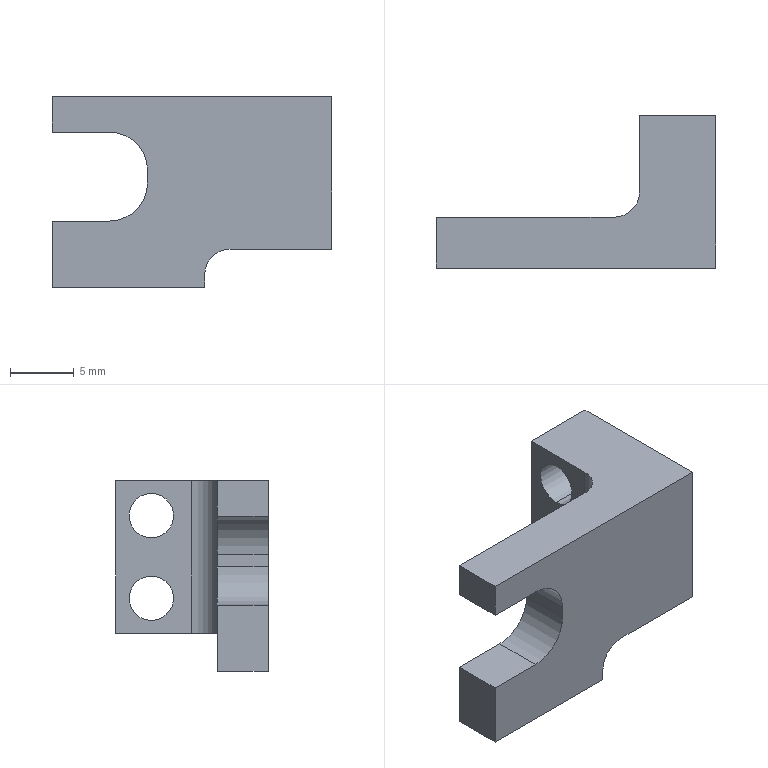Part | NX | features BREP 1 | 1 solid | 22 faces | box 22 x 12 x 15 mm | volume 1480 mm3 | plane 14 | cylinder 8 | commonest cylinder face diameters 3.5 x4 4 x2 6 x2
STEP:
#1=CARTESIAN_POINT('',(-769.249,20.164,1.));
#2=VERTEX_POINT('',#1);
#3=CARTESIAN_POINT('',(-769.249,20.164,4.5));
#4=VERTEX_POINT('',#3);
#5=CARTESIAN_POINT('',(-769.249,20.164,2.75));
#6=DIRECTION('',(-1.,0.,0.));
#7=DIRECTION('',(0.,0.,1.));
#8=AXIS2_PLACEMENT_3D('',#5,#6,#7);
#9=CIRCLE('',#8,1.75);
#10=EDGE_CURVE('',#2,#4,#9,.T.);
#11=ORIENTED_EDGE('',*,*,#10,.F.);
#12=CARTESIAN_POINT('',(-775.249,20.164,1.));
#13=VERTEX_POINT('',#12);
#14=CARTESIAN_POINT('',(-769.249,20.164,1.));
#15=DIRECTION('',(-1.,0.,0.));
#16=VECTOR('',#15,1000.);
#17=LINE('',#14,#16);
#18=EDGE_CURVE('',#13,#2,#17,.F.);
#19=ORIENTED_EDGE('',*,*,#18,.F.);
#20=CARTESIAN_POINT('',(-775.249,20.164,4.5));
#21=VERTEX_POINT('',#20);
#22=CARTESIAN_POINT('',(-775.249,20.164,2.75));
#23=DIRECTION('',(-1.,0.,0.));
#24=DIRECTION('',(0.,0.,1.));
#25=AXIS2_PLACEMENT_3D('',#22,#23,#24);
#26=CIRCLE('',#25,1.75);
#27=EDGE_CURVE('',#13,#21,#26,.T.);
#28=ORIENTED_EDGE('',*,*,#27,.T.);
#29=CARTESIAN_POINT('',(-769.249,20.164,4.5));
#30=DIRECTION('',(-1.,0.,0.));
#31=VECTOR('',#30,1000.);
#32=LINE('',#29,#31);
#33=EDGE_CURVE('',#21,#4,#32,.F.);
#34=ORIENTED_EDGE('',*,*,#33,.T.);
#35=EDGE_LOOP('',(#11,#19,#28,#34));
#36=FACE_BOUND('',#35,.T.);
#37=CARTESIAN_POINT('',(-769.249,20.164,2.75));
#38=DIRECTION('',(-1.,0.,0.));
#39=DIRECTION('',(0.,0.,1.));
#40=AXIS2_PLACEMENT_3D('',#37,#38,#39);
#41=CYLINDRICAL_SURFACE('',#40,1.75);
#42=ADVANCED_FACE('',(#36),#41,.F.);
#43=CARTESIAN_POINT('',(-769.249,20.164,7.5));
#44=VERTEX_POINT('',#43);
#45=CARTESIAN_POINT('',(-769.249,20.164,11.));
#46=VERTEX_POINT('',#45);
#47=CARTESIAN_POINT('',(-769.249,20.164,9.25));
#48=DIRECTION('',(-1.,0.,0.));
#49=DIRECTION('',(0.,0.,1.));
#50=AXIS2_PLACEMENT_3D('',#47,#48,#49);
#51=CIRCLE('',#50,1.75);
#52=EDGE_CURVE('',#44,#46,#51,.T.);
#53=ORIENTED_EDGE('',*,*,#52,.F.);
#54=CARTESIAN_POINT('',(-775.249,20.164,7.5));
#55=VERTEX_POINT('',#54);
#56=CARTESIAN_POINT('',(-769.249,20.164,7.5));
#57=DIRECTION('',(-1.,0.,0.));
#58=VECTOR('',#57,1000.);
#59=LINE('',#56,#58);
#60=EDGE_CURVE('',#55,#44,#59,.F.);
#61=ORIENTED_EDGE('',*,*,#60,.F.);
#62=CARTESIAN_POINT('',(-775.249,20.164,11.));
#63=VERTEX_POINT('',#62);
#64=CARTESIAN_POINT('',(-775.249,20.164,9.25));
#65=DIRECTION('',(-1.,0.,0.));
#66=DIRECTION('',(0.,0.,1.));
#67=AXIS2_PLACEMENT_3D('',#64,#65,#66);
#68=CIRCLE('',#67,1.75);
#69=EDGE_CURVE('',#55,#63,#68,.T.);
#70=ORIENTED_EDGE('',*,*,#69,.T.);
#71=CARTESIAN_POINT('',(-769.249,20.164,11.));
#72=DIRECTION('',(-1.,0.,0.));
#73=VECTOR('',#72,1000.);
#74=LINE('',#71,#73);
#75=EDGE_CURVE('',#63,#46,#74,.F.);
#76=ORIENTED_EDGE('',*,*,#75,.T.);
#77=EDGE_LOOP('',(#53,#61,#70,#76));
#78=FACE_BOUND('',#77,.T.);
#79=CARTESIAN_POINT('',(-769.249,20.164,9.25));
#80=DIRECTION('',(-1.,0.,0.));
#81=DIRECTION('',(0.,0.,1.));
#82=AXIS2_PLACEMENT_3D('',#79,#80,#81);
#83=CYLINDRICAL_SURFACE('',#82,1.75);
#84=ADVANCED_FACE('',(#78),#83,.F.);
#85=CARTESIAN_POINT('',(-791.249,10.964,9.213));
#86=VERTEX_POINT('',#85);
#87=CARTESIAN_POINT('',(-791.249,14.964,9.213));
#88=VERTEX_POINT('',#87);
#89=CARTESIAN_POINT('',(-791.249,14.964,9.213));
#90=DIRECTION('',(0.,1.,0.));
#91=VECTOR('',#90,1000.);
#92=LINE('',#89,#91);
#93=EDGE_CURVE('',#86,#88,#92,.T.);
#94=ORIENTED_EDGE('',*,*,#93,.F.);
#95=CARTESIAN_POINT('',(-791.249,10.964,12.));
#96=VERTEX_POINT('',#95);
#97=CARTESIAN_POINT('',(-791.249,10.964,12.));
#98=DIRECTION('',(0.,0.,1.));
#99=VECTOR('',#98,1000.);
#100=LINE('',#97,#99);
#101=EDGE_CURVE('',#86,#96,#100,.T.);
#102=ORIENTED_EDGE('',*,*,#101,.T.);
#103=CARTESIAN_POINT('',(-791.249,14.964,12.));
#104=VERTEX_POINT('',#103);
#105=CARTESIAN_POINT('',(-791.249,10.964,12.));
#106=DIRECTION('',(0.,1.,0.));
#107=VECTOR('',#106,1000.);
#108=LINE('',#105,#107);
#109=EDGE_CURVE('',#96,#104,#108,.T.);
#110=ORIENTED_EDGE('',*,*,#109,.T.);
#111=CARTESIAN_POINT('',(-791.249,14.964,12.));
#112=DIRECTION('',(0.,0.,-1.));
#113=VECTOR('',#112,1000.);
#114=LINE('',#111,#113);
#115=EDGE_CURVE('',#104,#88,#114,.T.);
#116=ORIENTED_EDGE('',*,*,#115,.T.);
#117=EDGE_LOOP('',(#94,#102,#110,#116));
#118=FACE_BOUND('',#117,.T.);
#119=CARTESIAN_POINT('',(-791.249,14.964,12.));
#120=DIRECTION('',(-1.,0.,0.));
#121=DIRECTION('',(0.,0.,1.));
#122=AXIS2_PLACEMENT_3D('',#119,#120,#121);
#123=PLANE('',#122);
#124=ADVANCED_FACE('',(#118),#123,.T.);
#125=CARTESIAN_POINT('',(-777.249,10.964,0.));
#126=VERTEX_POINT('',#125);
#127=CARTESIAN_POINT('',(-769.249,10.964,0.));
#128=VERTEX_POINT('',#127);
#129=CARTESIAN_POINT('',(-769.249,10.964,0.));
#130=DIRECTION('',(1.,0.,0.));
#131=VECTOR('',#130,1000.);
#132=LINE('',#129,#131);
#133=EDGE_CURVE('',#126,#128,#132,.T.);
#134=ORIENTED_EDGE('',*,*,#133,.F.);
#135=CARTESIAN_POINT('',(-777.249,14.964,0.));
#136=VERTEX_POINT('',#135);
#137=CARTESIAN_POINT('',(-777.249,14.964,0.));
#138=DIRECTION('',(0.,1.,0.));
#139=VECTOR('',#138,1000.);
#140=LINE('',#137,#139);
#141=EDGE_CURVE('',#126,#136,#140,.T.);
#142=ORIENTED_EDGE('',*,*,#141,.T.);
#143=CARTESIAN_POINT('',(-775.249,16.964,0.));
#144=VERTEX_POINT('',#143);
#145=CARTESIAN_POINT('',(-777.249,16.964,0.));
#146=DIRECTION('',(0.,0.,1.));
#147=DIRECTION('',(-1.,0.,0.));
#148=AXIS2_PLACEMENT_3D('',#145,#146,#147);
#149=CIRCLE('',#148,2.);
#150=EDGE_CURVE('',#136,#144,#149,.T.);
#151=ORIENTED_EDGE('',*,*,#150,.T.);
#152=CARTESIAN_POINT('',(-775.249,22.964,0.));
#153=VERTEX_POINT('',#152);
#154=CARTESIAN_POINT('',(-775.249,22.964,0.));
#155=DIRECTION('',(0.,-1.,0.));
#156=VECTOR('',#155,1000.);
#157=LINE('',#154,#156);
#158=EDGE_CURVE('',#153,#144,#157,.T.);
#159=ORIENTED_EDGE('',*,*,#158,.F.);
#160=CARTESIAN_POINT('',(-769.249,22.964,0.));
#161=VERTEX_POINT('',#160);
#162=CARTESIAN_POINT('',(-769.249,22.964,0.));
#163=DIRECTION('',(-1.,0.,0.));
#164=VECTOR('',#163,1000.);
#165=LINE('',#162,#164);
#166=EDGE_CURVE('',#161,#153,#165,.T.);
#167=ORIENTED_EDGE('',*,*,#166,.F.);
#168=CARTESIAN_POINT('',(-769.249,22.964,0.));
#169=DIRECTION('',(0.,1.,0.));
#170=VECTOR('',#169,1000.);
#171=LINE('',#168,#170);
#172=EDGE_CURVE('',#128,#161,#171,.T.);
#173=ORIENTED_EDGE('',*,*,#172,.F.);
#174=EDGE_LOOP('',(#134,#142,#151,#159,#167,#173));
#175=FACE_BOUND('',#174,.T.);
#176=CARTESIAN_POINT('',(-769.249,10.964,0.));
#177=DIRECTION('',(0.,0.,-1.));
#178=DIRECTION('',(0.,-1.,0.));
#179=AXIS2_PLACEMENT_3D('',#176,#177,#178);
#180=PLANE('',#179);
#181=ADVANCED_FACE('',(#175),#180,.T.);
#182=ORIENTED_EDGE('',*,*,#158,.T.);
#183=CARTESIAN_POINT('',(-775.249,16.964,12.));
#184=VERTEX_POINT('',#183);
#185=CARTESIAN_POINT('',(-775.249,16.964,12.));
#186=DIRECTION('',(0.,0.,1.));
#187=VECTOR('',#186,1000.);
#188=LINE('',#185,#187);
#189=EDGE_CURVE('',#144,#184,#188,.T.);
#190=ORIENTED_EDGE('',*,*,#189,.T.);
#191=CARTESIAN_POINT('',(-775.249,22.964,12.));
#192=VERTEX_POINT('',#191);
#193=CARTESIAN_POINT('',(-775.249,22.964,12.));
#194=DIRECTION('',(0.,-1.,0.));
#195=VECTOR('',#194,1000.);
#196=LINE('',#193,#195);
#197=EDGE_CURVE('',#192,#184,#196,.T.);
#198=ORIENTED_EDGE('',*,*,#197,.F.);
#199=CARTESIAN_POINT('',(-775.249,22.964,12.));
#200=DIRECTION('',(0.,0.,-1.));
#201=VECTOR('',#200,1000.);
#202=LINE('',#199,#201);
#203=EDGE_CURVE('',#192,#153,#202,.T.);
#204=ORIENTED_EDGE('',*,*,#203,.T.);
#205=EDGE_LOOP('',(#182,#190,#198,#204));
#206=FACE_BOUND('',#205,.T.);
#207=CARTESIAN_POINT('',(-775.249,20.164,2.75));
#208=DIRECTION('',(-1.,0.,0.));
#209=DIRECTION('',(0.,0.,1.));
#210=AXIS2_PLACEMENT_3D('',#207,#208,#209);
#211=CIRCLE('',#210,1.75);
#212=EDGE_CURVE('',#21,#13,#211,.T.);
#213=ORIENTED_EDGE('',*,*,#212,.F.);
#214=ORIENTED_EDGE('',*,*,#27,.F.);
#215=EDGE_LOOP('',(#213,#214));
#216=FACE_BOUND('',#215,.T.);
#217=CARTESIAN_POINT('',(-775.249,20.164,9.25));
#218=DIRECTION('',(-1.,0.,0.));
#219=DIRECTION('',(0.,0.,1.));
#220=AXIS2_PLACEMENT_3D('',#217,#218,#219);
#221=CIRCLE('',#220,1.75);
#222=EDGE_CURVE('',#63,#55,#221,.T.);
#223=ORIENTED_EDGE('',*,*,#222,.F.);
#224=ORIENTED_EDGE('',*,*,#69,.F.);
#225=EDGE_LOOP('',(#223,#224));
#226=FACE_BOUND('',#225,.T.);
#227=CARTESIAN_POINT('',(-775.249,22.964,12.));
#228=DIRECTION('',(1.,0.,0.));
#229=DIRECTION('',(0.,1.,0.));
#230=AXIS2_PLACEMENT_3D('',#227,#228,#229);
#231=PLANE('',#230);
#232=ADVANCED_FACE('',(#206,#216,#226),#231,.F.);
#233=ORIENTED_EDGE('',*,*,#172,.T.);
#234=CARTESIAN_POINT('',(-769.249,22.964,12.));
#235=VERTEX_POINT('',#234);
#236=CARTESIAN_POINT('',(-769.249,22.964,12.));
#237=DIRECTION('',(0.,0.,-1.));
#238=VECTOR('',#237,1000.);
#239=LINE('',#236,#238);
#240=EDGE_CURVE('',#235,#161,#239,.T.);
#241=ORIENTED_EDGE('',*,*,#240,.F.);
#242=CARTESIAN_POINT('',(-769.249,10.964,12.));
#243=VERTEX_POINT('',#242);
#244=CARTESIAN_POINT('',(-769.249,22.964,12.));
#245=DIRECTION('',(0.,1.,0.));
#246=VECTOR('',#245,1000.);
#247=LINE('',#244,#246);
#248=EDGE_CURVE('',#243,#235,#247,.T.);
#249=ORIENTED_EDGE('',*,*,#248,.F.);
#250=CARTESIAN_POINT('',(-769.249,10.964,12.));
#251=DIRECTION('',(0.,0.,-1.));
#252=VECTOR('',#251,1000.);
#253=LINE('',#250,#252);
#254=EDGE_CURVE('',#243,#128,#253,.T.);
#255=ORIENTED_EDGE('',*,*,#254,.T.);
#256=EDGE_LOOP('',(#233,#241,#249,#255));
#257=FACE_BOUND('',#256,.T.);
#258=CARTESIAN_POINT('',(-769.249,20.164,2.75));
#259=DIRECTION('',(-1.,0.,0.));
#260=DIRECTION('',(0.,0.,1.));
#261=AXIS2_PLACEMENT_3D('',#258,#259,#260);
#262=CIRCLE('',#261,1.75);
#263=EDGE_CURVE('',#4,#2,#262,.T.);
#264=ORIENTED_EDGE('',*,*,#263,.T.);
#265=ORIENTED_EDGE('',*,*,#10,.T.);
#266=EDGE_LOOP('',(#264,#265));
#267=FACE_BOUND('',#266,.T.);
#268=CARTESIAN_POINT('',(-769.249,20.164,9.25));
#269=DIRECTION('',(-1.,0.,0.));
#270=DIRECTION('',(0.,0.,1.));
#271=AXIS2_PLACEMENT_3D('',#268,#269,#270);
#272=CIRCLE('',#271,1.75);
#273=EDGE_CURVE('',#46,#44,#272,.T.);
#274=ORIENTED_EDGE('',*,*,#273,.T.);
#275=ORIENTED_EDGE('',*,*,#52,.T.);
#276=EDGE_LOOP('',(#274,#275));
#277=FACE_BOUND('',#276,.T.);
#278=CARTESIAN_POINT('',(-769.249,22.964,12.));
#279=DIRECTION('',(-1.,0.,0.));
#280=DIRECTION('',(0.,0.,1.));
#281=AXIS2_PLACEMENT_3D('',#278,#279,#280);
#282=PLANE('',#281);
#283=ADVANCED_FACE('',(#257,#267,#277),#282,.F.);
#284=ORIENTED_EDGE('',*,*,#166,.T.);
#285=ORIENTED_EDGE('',*,*,#203,.F.);
#286=CARTESIAN_POINT('',(-769.249,22.964,12.));
#287=DIRECTION('',(-1.,0.,0.));
#288=VECTOR('',#287,1000.);
#289=LINE('',#286,#288);
#290=EDGE_CURVE('',#235,#192,#289,.T.);
#291=ORIENTED_EDGE('',*,*,#290,.F.);
#292=ORIENTED_EDGE('',*,*,#240,.T.);
#293=EDGE_LOOP('',(#284,#285,#291,#292));
#294=FACE_BOUND('',#293,.T.);
#295=CARTESIAN_POINT('',(-769.249,22.964,12.));
#296=DIRECTION('',(0.,-1.,0.));
#297=DIRECTION('',(0.,0.,-1.));
#298=AXIS2_PLACEMENT_3D('',#295,#296,#297);
#299=PLANE('',#298);
#300=ADVANCED_FACE('',(#294),#299,.F.);
#301=ORIENTED_EDGE('',*,*,#101,.F.);
#302=CARTESIAN_POINT('',(-786.749,10.964,9.213));
#303=VERTEX_POINT('',#302);
#304=CARTESIAN_POINT('',(-769.249,10.964,9.213));
#305=DIRECTION('',(1.,0.,0.));
#306=VECTOR('',#305,1000.);
#307=LINE('',#304,#306);
#308=EDGE_CURVE('',#86,#303,#307,.T.);
#309=ORIENTED_EDGE('',*,*,#308,.T.);
#310=CARTESIAN_POINT('',(-783.749,10.964,6.213));
#311=VERTEX_POINT('',#310);
#312=CARTESIAN_POINT('',(-786.749,10.964,6.213));
#313=DIRECTION('',(0.,1.,0.));
#314=DIRECTION('',(-1.,0.,0.));
#315=AXIS2_PLACEMENT_3D('',#312,#313,#314);
#316=CIRCLE('',#315,3.);
#317=EDGE_CURVE('',#303,#311,#316,.T.);
#318=ORIENTED_EDGE('',*,*,#317,.T.);
#319=CARTESIAN_POINT('',(-783.749,10.964,5.213));
#320=VERTEX_POINT('',#319);
#321=CARTESIAN_POINT('',(-783.749,10.964,12.));
#322=DIRECTION('',(0.,0.,-1.));
#323=VECTOR('',#322,1000.);
#324=LINE('',#321,#323);
#325=EDGE_CURVE('',#311,#320,#324,.T.);
#326=ORIENTED_EDGE('',*,*,#325,.T.);
#327=CARTESIAN_POINT('',(-786.749,10.964,2.213));
#328=VERTEX_POINT('',#327);
#329=CARTESIAN_POINT('',(-786.749,10.964,5.213));
#330=DIRECTION('',(0.,1.,0.));
#331=DIRECTION('',(-1.,0.,0.));
#332=AXIS2_PLACEMENT_3D('',#329,#330,#331);
#333=CIRCLE('',#332,3.);
#334=EDGE_CURVE('',#320,#328,#333,.T.);
#335=ORIENTED_EDGE('',*,*,#334,.T.);
#336=CARTESIAN_POINT('',(-791.249,10.964,2.213));
#337=VERTEX_POINT('',#336);
#338=CARTESIAN_POINT('',(-769.249,10.964,2.213));
#339=DIRECTION('',(-1.,0.,0.));
#340=VECTOR('',#339,1000.);
#341=LINE('',#338,#340);
#342=EDGE_CURVE('',#328,#337,#341,.T.);
#343=ORIENTED_EDGE('',*,*,#342,.T.);
#344=CARTESIAN_POINT('',(-791.249,10.964,-3.));
#345=VERTEX_POINT('',#344);
#346=CARTESIAN_POINT('',(-791.249,10.964,12.));
#347=DIRECTION('',(0.,0.,1.));
#348=VECTOR('',#347,1000.);
#349=LINE('',#346,#348);
#350=EDGE_CURVE('',#345,#337,#349,.T.);
#351=ORIENTED_EDGE('',*,*,#350,.F.);
#352=CARTESIAN_POINT('',(-779.249,10.964,-3.));
#353=VERTEX_POINT('',#352);
#354=CARTESIAN_POINT('',(-791.249,10.964,-3.));
#355=DIRECTION('',(1.,0.,0.));
#356=VECTOR('',#355,1000.);
#357=LINE('',#354,#356);
#358=EDGE_CURVE('',#345,#353,#357,.T.);
#359=ORIENTED_EDGE('',*,*,#358,.T.);
#360=CARTESIAN_POINT('',(-779.249,10.964,-2.));
#361=VERTEX_POINT('',#360);
#362=CARTESIAN_POINT('',(-779.249,10.964,0.));
#363=DIRECTION('',(0.,0.,1.));
#364=VECTOR('',#363,1000.);
#365=LINE('',#362,#364);
#366=EDGE_CURVE('',#353,#361,#365,.T.);
#367=ORIENTED_EDGE('',*,*,#366,.T.);
#368=CARTESIAN_POINT('',(-777.249,10.964,-2.));
#369=DIRECTION('',(0.,1.,0.));
#370=DIRECTION('',(-1.,0.,0.));
#371=AXIS2_PLACEMENT_3D('',#368,#369,#370);
#372=CIRCLE('',#371,2.);
#373=EDGE_CURVE('',#361,#126,#372,.T.);
#374=ORIENTED_EDGE('',*,*,#373,.T.);
#375=ORIENTED_EDGE('',*,*,#133,.T.);
#376=ORIENTED_EDGE('',*,*,#254,.F.);
#377=CARTESIAN_POINT('',(-769.249,10.964,12.));
#378=DIRECTION('',(1.,0.,0.));
#379=VECTOR('',#378,1000.);
#380=LINE('',#377,#379);
#381=EDGE_CURVE('',#96,#243,#380,.T.);
#382=ORIENTED_EDGE('',*,*,#381,.F.);
#383=EDGE_LOOP('',(#301,#309,#318,#326,#335,#343,#351,#359,#367,#374,#375,#376,#382));
#384=FACE_BOUND('',#383,.T.);
#385=CARTESIAN_POINT('',(-769.249,10.964,12.));
#386=DIRECTION('',(0.,1.,0.));
#387=DIRECTION('',(1.,0.,0.));
#388=AXIS2_PLACEMENT_3D('',#385,#386,#387);
#389=PLANE('',#388);
#390=ADVANCED_FACE('',(#384),#389,.F.);
#391=ORIENTED_EDGE('',*,*,#248,.T.);
#392=ORIENTED_EDGE('',*,*,#290,.T.);
#393=ORIENTED_EDGE('',*,*,#197,.T.);
#394=CARTESIAN_POINT('',(-777.249,14.964,12.));
#395=VERTEX_POINT('',#394);
#396=CARTESIAN_POINT('',(-777.249,16.964,12.));
#397=DIRECTION('',(0.,0.,-1.));
#398=DIRECTION('',(-1.,0.,0.));
#399=AXIS2_PLACEMENT_3D('',#396,#397,#398);
#400=CIRCLE('',#399,2.);
#401=EDGE_CURVE('',#184,#395,#400,.T.);
#402=ORIENTED_EDGE('',*,*,#401,.T.);
#403=CARTESIAN_POINT('',(-791.249,14.964,12.));
#404=DIRECTION('',(1.,0.,0.));
#405=VECTOR('',#404,1000.);
#406=LINE('',#403,#405);
#407=EDGE_CURVE('',#104,#395,#406,.T.);
#408=ORIENTED_EDGE('',*,*,#407,.F.);
#409=ORIENTED_EDGE('',*,*,#109,.F.);
#410=ORIENTED_EDGE('',*,*,#381,.T.);
#411=EDGE_LOOP('',(#391,#392,#393,#402,#408,#409,#410));
#412=FACE_BOUND('',#411,.T.);
#413=CARTESIAN_POINT('',(-769.249,10.964,12.));
#414=DIRECTION('',(0.,0.,-1.));
#415=DIRECTION('',(0.,-1.,0.));
#416=AXIS2_PLACEMENT_3D('',#413,#414,#415);
#417=PLANE('',#416);
#418=ADVANCED_FACE('',(#412),#417,.F.);
#419=CARTESIAN_POINT('',(-783.749,14.964,6.213));
#420=VERTEX_POINT('',#419);
#421=CARTESIAN_POINT('',(-783.749,14.964,5.213));
#422=VERTEX_POINT('',#421);
#423=CARTESIAN_POINT('',(-783.749,14.964,9.213));
#424=DIRECTION('',(0.,0.,-1.));
#425=VECTOR('',#424,1000.);
#426=LINE('',#423,#425);
#427=EDGE_CURVE('',#420,#422,#426,.T.);
#428=ORIENTED_EDGE('',*,*,#427,.F.);
#429=CARTESIAN_POINT('',(-786.749,14.964,9.213));
#430=VERTEX_POINT('',#429);
#431=CARTESIAN_POINT('',(-786.749,14.964,6.213));
#432=DIRECTION('',(0.,-1.,0.));
#433=DIRECTION('',(0.,0.,-1.));
#434=AXIS2_PLACEMENT_3D('',#431,#432,#433);
#435=CIRCLE('',#434,3.);
#436=EDGE_CURVE('',#420,#430,#435,.T.);
#437=ORIENTED_EDGE('',*,*,#436,.T.);
#438=CARTESIAN_POINT('',(-783.749,14.964,9.213));
#439=DIRECTION('',(1.,0.,0.));
#440=VECTOR('',#439,1000.);
#441=LINE('',#438,#440);
#442=EDGE_CURVE('',#88,#430,#441,.T.);
#443=ORIENTED_EDGE('',*,*,#442,.F.);
#444=ORIENTED_EDGE('',*,*,#115,.F.);
#445=ORIENTED_EDGE('',*,*,#407,.T.);
#446=CARTESIAN_POINT('',(-777.249,14.964,0.));
#447=DIRECTION('',(0.,0.,-1.));
#448=VECTOR('',#447,1000.);
#449=LINE('',#446,#448);
#450=EDGE_CURVE('',#395,#136,#449,.T.);
#451=ORIENTED_EDGE('',*,*,#450,.T.);
#452=CARTESIAN_POINT('',(-779.249,14.964,-2.));
#453=VERTEX_POINT('',#452);
#454=CARTESIAN_POINT('',(-777.249,14.964,-2.));
#455=DIRECTION('',(0.,-1.,0.));
#456=DIRECTION('',(0.,0.,-1.));
#457=AXIS2_PLACEMENT_3D('',#454,#455,#456);
#458=CIRCLE('',#457,2.);
#459=EDGE_CURVE('',#136,#453,#458,.T.);
#460=ORIENTED_EDGE('',*,*,#459,.T.);
#461=CARTESIAN_POINT('',(-779.249,14.964,-3.));
#462=VERTEX_POINT('',#461);
#463=CARTESIAN_POINT('',(-779.249,14.964,0.));
#464=DIRECTION('',(0.,0.,-1.));
#465=VECTOR('',#464,1000.);
#466=LINE('',#463,#465);
#467=EDGE_CURVE('',#453,#462,#466,.T.);
#468=ORIENTED_EDGE('',*,*,#467,.T.);
#469=CARTESIAN_POINT('',(-791.249,14.964,-3.));
#470=VERTEX_POINT('',#469);
#471=CARTESIAN_POINT('',(-791.249,14.964,-3.));
#472=DIRECTION('',(-1.,0.,0.));
#473=VECTOR('',#472,1000.);
#474=LINE('',#471,#473);
#475=EDGE_CURVE('',#462,#470,#474,.T.);
#476=ORIENTED_EDGE('',*,*,#475,.T.);
#477=CARTESIAN_POINT('',(-791.249,14.964,2.213));
#478=VERTEX_POINT('',#477);
#479=CARTESIAN_POINT('',(-791.249,14.964,12.));
#480=DIRECTION('',(0.,0.,-1.));
#481=VECTOR('',#480,1000.);
#482=LINE('',#479,#481);
#483=EDGE_CURVE('',#478,#470,#482,.T.);
#484=ORIENTED_EDGE('',*,*,#483,.F.);
#485=CARTESIAN_POINT('',(-786.749,14.964,2.213));
#486=VERTEX_POINT('',#485);
#487=CARTESIAN_POINT('',(-783.749,14.964,2.213));
#488=DIRECTION('',(-1.,0.,0.));
#489=VECTOR('',#488,1000.);
#490=LINE('',#487,#489);
#491=EDGE_CURVE('',#486,#478,#490,.T.);
#492=ORIENTED_EDGE('',*,*,#491,.F.);
#493=CARTESIAN_POINT('',(-786.749,14.964,5.213));
#494=DIRECTION('',(0.,-1.,0.));
#495=DIRECTION('',(0.,0.,-1.));
#496=AXIS2_PLACEMENT_3D('',#493,#494,#495);
#497=CIRCLE('',#496,3.);
#498=EDGE_CURVE('',#486,#422,#497,.T.);
#499=ORIENTED_EDGE('',*,*,#498,.T.);
#500=EDGE_LOOP('',(#428,#437,#443,#444,#445,#451,#460,#468,#476,#484,#492,#499));
#501=FACE_BOUND('',#500,.T.);
#502=CARTESIAN_POINT('',(-791.249,14.964,12.));
#503=DIRECTION('',(0.,-1.,0.));
#504=DIRECTION('',(-1.,0.,0.));
#505=AXIS2_PLACEMENT_3D('',#502,#503,#504);
#506=PLANE('',#505);
#507=ADVANCED_FACE('',(#501),#506,.F.);
#508=CARTESIAN_POINT('',(-791.249,14.964,2.213));
#509=DIRECTION('',(0.,-1.,0.));
#510=VECTOR('',#509,1000.);
#511=LINE('',#508,#510);
#512=EDGE_CURVE('',#478,#337,#511,.T.);
#513=ORIENTED_EDGE('',*,*,#512,.F.);
#514=ORIENTED_EDGE('',*,*,#483,.T.);
#515=CARTESIAN_POINT('',(-791.249,-1.405,-3.));
#516=DIRECTION('',(0.,1.,0.));
#517=VECTOR('',#516,1000.);
#518=LINE('',#515,#517);
#519=EDGE_CURVE('',#345,#470,#518,.T.);
#520=ORIENTED_EDGE('',*,*,#519,.F.);
#521=ORIENTED_EDGE('',*,*,#350,.T.);
#522=EDGE_LOOP('',(#513,#514,#520,#521));
#523=FACE_BOUND('',#522,.T.);
#524=CARTESIAN_POINT('',(-791.249,14.964,12.));
#525=DIRECTION('',(-1.,0.,0.));
#526=DIRECTION('',(0.,0.,1.));
#527=AXIS2_PLACEMENT_3D('',#524,#525,#526);
#528=PLANE('',#527);
#529=ADVANCED_FACE('',(#523),#528,.T.);
#530=ORIENTED_EDGE('',*,*,#401,.F.);
#531=ORIENTED_EDGE('',*,*,#189,.F.);
#532=ORIENTED_EDGE('',*,*,#150,.F.);
#533=ORIENTED_EDGE('',*,*,#450,.F.);
#534=EDGE_LOOP('',(#530,#531,#532,#533));
#535=FACE_BOUND('',#534,.T.);
#536=CARTESIAN_POINT('',(-777.249,16.964,12.));
#537=DIRECTION('',(0.,0.,1.));
#538=DIRECTION('',(0.,-1.,0.));
#539=AXIS2_PLACEMENT_3D('',#536,#537,#538);
#540=CYLINDRICAL_SURFACE('',#539,2.);
#541=ADVANCED_FACE('',(#535),#540,.F.);
#542=ORIENTED_EDGE('',*,*,#358,.F.);
#543=ORIENTED_EDGE('',*,*,#519,.T.);
#544=ORIENTED_EDGE('',*,*,#475,.F.);
#545=CARTESIAN_POINT('',(-779.249,-1.405,-3.));
#546=DIRECTION('',(0.,1.,0.));
#547=VECTOR('',#546,1000.);
#548=LINE('',#545,#547);
#549=EDGE_CURVE('',#353,#462,#548,.T.);
#550=ORIENTED_EDGE('',*,*,#549,.F.);
#551=EDGE_LOOP('',(#542,#543,#544,#550));
#552=FACE_BOUND('',#551,.T.);
#553=CARTESIAN_POINT('',(-791.249,-1.405,-3.));
#554=DIRECTION('',(0.,0.,-1.));
#555=DIRECTION('',(0.,-1.,0.));
#556=AXIS2_PLACEMENT_3D('',#553,#554,#555);
#557=PLANE('',#556);
#558=ADVANCED_FACE('',(#552),#557,.T.);
#559=ORIENTED_EDGE('',*,*,#467,.F.);
#560=CARTESIAN_POINT('',(-779.249,10.964,-2.));
#561=DIRECTION('',(0.,-1.,0.));
#562=VECTOR('',#561,1000.);
#563=LINE('',#560,#562);
#564=EDGE_CURVE('',#453,#361,#563,.T.);
#565=ORIENTED_EDGE('',*,*,#564,.T.);
#566=ORIENTED_EDGE('',*,*,#366,.F.);
#567=ORIENTED_EDGE('',*,*,#549,.T.);
#568=EDGE_LOOP('',(#559,#565,#566,#567));
#569=FACE_BOUND('',#568,.T.);
#570=CARTESIAN_POINT('',(-779.249,-1.405,0.));
#571=DIRECTION('',(1.,0.,0.));
#572=DIRECTION('',(0.,1.,0.));
#573=AXIS2_PLACEMENT_3D('',#570,#571,#572);
#574=PLANE('',#573);
#575=ADVANCED_FACE('',(#569),#574,.T.);
#576=ORIENTED_EDGE('',*,*,#427,.T.);
#577=CARTESIAN_POINT('',(-783.749,10.964,5.213));
#578=DIRECTION('',(0.,-1.,0.));
#579=VECTOR('',#578,1000.);
#580=LINE('',#577,#579);
#581=EDGE_CURVE('',#422,#320,#580,.T.);
#582=ORIENTED_EDGE('',*,*,#581,.T.);
#583=ORIENTED_EDGE('',*,*,#325,.F.);
#584=CARTESIAN_POINT('',(-783.749,14.964,6.213));
#585=DIRECTION('',(0.,1.,0.));
#586=VECTOR('',#585,1000.);
#587=LINE('',#584,#586);
#588=EDGE_CURVE('',#311,#420,#587,.T.);
#589=ORIENTED_EDGE('',*,*,#588,.T.);
#590=EDGE_LOOP('',(#576,#582,#583,#589));
#591=FACE_BOUND('',#590,.T.);
#592=CARTESIAN_POINT('',(-783.749,10.964,9.213));
#593=DIRECTION('',(1.,0.,0.));
#594=DIRECTION('',(0.,1.,0.));
#595=AXIS2_PLACEMENT_3D('',#592,#593,#594);
#596=PLANE('',#595);
#597=ADVANCED_FACE('',(#591),#596,.F.);
#598=ORIENTED_EDGE('',*,*,#442,.T.);
#599=CARTESIAN_POINT('',(-786.749,10.964,9.213));
#600=DIRECTION('',(0.,-1.,0.));
#601=VECTOR('',#600,1000.);
#602=LINE('',#599,#601);
#603=EDGE_CURVE('',#430,#303,#602,.T.);
#604=ORIENTED_EDGE('',*,*,#603,.T.);
#605=ORIENTED_EDGE('',*,*,#308,.F.);
#606=ORIENTED_EDGE('',*,*,#93,.T.);
#607=EDGE_LOOP('',(#598,#604,#605,#606));
#608=FACE_BOUND('',#607,.T.);
#609=CARTESIAN_POINT('',(-783.749,10.964,9.213));
#610=DIRECTION('',(0.,0.,1.));
#611=DIRECTION('',(1.,0.,0.));
#612=AXIS2_PLACEMENT_3D('',#609,#610,#611);
#613=PLANE('',#612);
#614=ADVANCED_FACE('',(#608),#613,.F.);
#615=ORIENTED_EDGE('',*,*,#342,.F.);
#616=CARTESIAN_POINT('',(-786.749,14.964,2.213));
#617=DIRECTION('',(0.,1.,0.));
#618=VECTOR('',#617,1000.);
#619=LINE('',#616,#618);
#620=EDGE_CURVE('',#328,#486,#619,.T.);
#621=ORIENTED_EDGE('',*,*,#620,.T.);
#622=ORIENTED_EDGE('',*,*,#491,.T.);
#623=ORIENTED_EDGE('',*,*,#512,.T.);
#624=EDGE_LOOP('',(#615,#621,#622,#623));
#625=FACE_BOUND('',#624,.T.);
#626=CARTESIAN_POINT('',(-783.749,10.964,2.213));
#627=DIRECTION('',(0.,0.,-1.));
#628=DIRECTION('',(-1.,0.,0.));
#629=AXIS2_PLACEMENT_3D('',#626,#627,#628);
#630=PLANE('',#629);
#631=ADVANCED_FACE('',(#625),#630,.F.);
#632=ORIENTED_EDGE('',*,*,#334,.F.);
#633=ORIENTED_EDGE('',*,*,#581,.F.);
#634=ORIENTED_EDGE('',*,*,#498,.F.);
#635=ORIENTED_EDGE('',*,*,#620,.F.);
#636=EDGE_LOOP('',(#632,#633,#634,#635));
#637=FACE_BOUND('',#636,.T.);
#638=CARTESIAN_POINT('',(-786.749,10.964,5.213));
#639=DIRECTION('',(0.,-1.,0.));
#640=DIRECTION('',(0.,0.,-1.));
#641=AXIS2_PLACEMENT_3D('',#638,#639,#640);
#642=CYLINDRICAL_SURFACE('',#641,3.);
#643=ADVANCED_FACE('',(#637),#642,.F.);
#644=ORIENTED_EDGE('',*,*,#317,.F.);
#645=ORIENTED_EDGE('',*,*,#603,.F.);
#646=ORIENTED_EDGE('',*,*,#436,.F.);
#647=ORIENTED_EDGE('',*,*,#588,.F.);
#648=EDGE_LOOP('',(#644,#645,#646,#647));
#649=FACE_BOUND('',#648,.T.);
#650=CARTESIAN_POINT('',(-786.749,10.964,6.213));
#651=DIRECTION('',(0.,-1.,0.));
#652=DIRECTION('',(0.,0.,-1.));
#653=AXIS2_PLACEMENT_3D('',#650,#651,#652);
#654=CYLINDRICAL_SURFACE('',#653,3.);
#655=ADVANCED_FACE('',(#649),#654,.F.);
#656=ORIENTED_EDGE('',*,*,#60,.T.);
#657=ORIENTED_EDGE('',*,*,#273,.F.);
#658=ORIENTED_EDGE('',*,*,#75,.F.);
#659=ORIENTED_EDGE('',*,*,#222,.T.);
#660=EDGE_LOOP('',(#656,#657,#658,#659));
#661=FACE_BOUND('',#660,.T.);
#662=CARTESIAN_POINT('',(-769.249,20.164,9.25));
#663=DIRECTION('',(-1.,0.,0.));
#664=DIRECTION('',(0.,0.,1.));
#665=AXIS2_PLACEMENT_3D('',#662,#663,#664);
#666=CYLINDRICAL_SURFACE('',#665,1.75);
#667=ADVANCED_FACE('',(#661),#666,.F.);
#668=ORIENTED_EDGE('',*,*,#18,.T.);
#669=ORIENTED_EDGE('',*,*,#263,.F.);
#670=ORIENTED_EDGE('',*,*,#33,.F.);
#671=ORIENTED_EDGE('',*,*,#212,.T.);
#672=EDGE_LOOP('',(#668,#669,#670,#671));
#673=FACE_BOUND('',#672,.T.);
#674=CARTESIAN_POINT('',(-769.249,20.164,2.75));
#675=DIRECTION('',(-1.,0.,0.));
#676=DIRECTION('',(0.,0.,1.));
#677=AXIS2_PLACEMENT_3D('',#674,#675,#676);
#678=CYLINDRICAL_SURFACE('',#677,1.75);
#679=ADVANCED_FACE('',(#673),#678,.F.);
#680=ORIENTED_EDGE('',*,*,#373,.F.);
#681=ORIENTED_EDGE('',*,*,#564,.F.);
#682=ORIENTED_EDGE('',*,*,#459,.F.);
#683=ORIENTED_EDGE('',*,*,#141,.F.);
#684=EDGE_LOOP('',(#680,#681,#682,#683));
#685=FACE_BOUND('',#684,.T.);
#686=CARTESIAN_POINT('',(-777.249,10.964,-2.));
#687=DIRECTION('',(0.,-1.,0.));
#688=DIRECTION('',(0.,0.,-1.));
#689=AXIS2_PLACEMENT_3D('',#686,#687,#688);
#690=CYLINDRICAL_SURFACE('',#689,2.);
#691=ADVANCED_FACE('',(#685),#690,.F.);
#692=CLOSED_SHELL('',(#42,#84,#124,#181,#232,#283,#300,#390,#418,#507,#529,#541,#558,#575,#597,#614,#631,#643,#655,#667,#679,#691));
#693=MANIFOLD_SOLID_BREP('',#692);
#694=(LENGTH_UNIT()NAMED_UNIT(*)SI_UNIT(.MILLI.,.METRE.));
#695=UNCERTAINTY_MEASURE_WITH_UNIT(LENGTH_MEASURE(0.00001),#694,'','');
#696=(NAMED_UNIT(*)PLANE_ANGLE_UNIT()SI_UNIT($,.RADIAN.));
#697=(NAMED_UNIT(*)SI_UNIT($,.STERADIAN.)SOLID_ANGLE_UNIT());
#698=(GEOMETRIC_REPRESENTATION_CONTEXT(3)GLOBAL_UNCERTAINTY_ASSIGNED_CONTEXT((#695))GLOBAL_UNIT_ASSIGNED_CONTEXT((#694,#696,#697))REPRESENTATION_CONTEXT('',''));
#699=ADVANCED_BREP_SHAPE_REPRESENTATION('',(#693),#698);